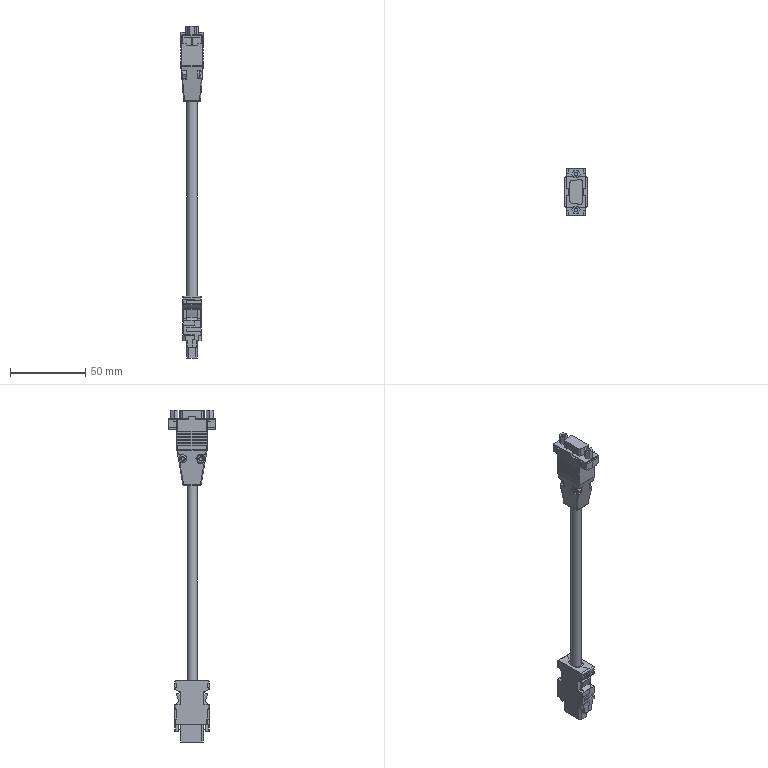Part | STEP file | BODYMSM_E-RAM6-S-640-ME30-C5 | 1 solid | 532 faces | box 14.9 x 31.1 x 221.16 mm | volume 25998 mm3 | plane 355 | cylinder 111 | cone 26 | torus 20 | sphere 12 | spline 8 | commonest cylinder face diameters 0.4 x51 2 x24 1 x20 3 x6 2.459 x2 5 x2